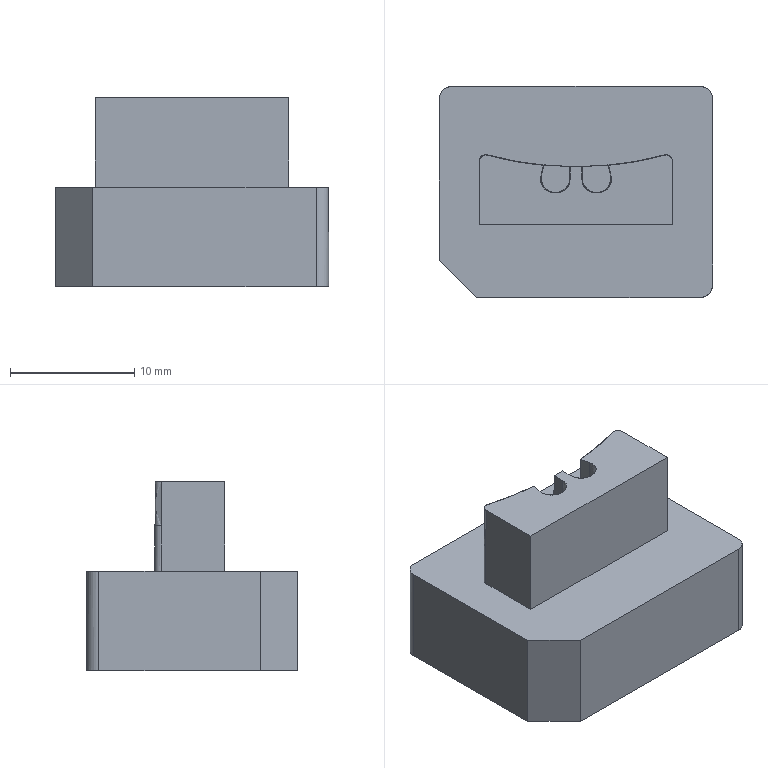NC program | PowerMill | posted by the shop | part box 22 x 17 x 15.232 mm
Lines 11891 to 12632 of 87032:
( TOOL ID   D10_1_1 )
( TOOL DIA. 10. TIP RAD 0 LENGTH 70.4 )
( Z = -.248 )
T3 M6
T10
G91 G28 Z0
G0 G90 G54
M08
S8500 M3
X0 Y0 M8
G43 Z11.802 H3
X-18.215 Y-5.282
Z.952
G1 Z-.248 F360
X-13.104 Y-3.978 F600
X13.103
X13.154 Y-3.766
X13.205 Y-3.487
X13.245 Y-3.182
X13.269 Y-2.829
X13.274 Y-2.625
X13.273 Y.169
X-13.273
Y2.529
X-13.26 Y2.854
X-13.232 Y3.17
X-13.175 Y3.546
X-13.12 Y3.806
X-13.057 Y4.058
X-12.979 Y4.315
X12.979
G0 Z11.802
X0 Y0
Z9.802
X-14.745 Y-16.901
Z-6.23
G1 Z-7.43 F360
X-11.441 Y-12.789 F600
X-1.912 Y-8.025
X-7.919 Y-8.023
X-8.202 Y-8.008
X-8.485 Y-7.978
X-8.768 Y-7.933
X-9.05 Y-7.872
X-9.333 Y-7.795
X-9.616 Y-7.701
X-9.951 Y-7.566
X-10.182 Y-7.458
X-10.464 Y-7.307
X-10.805 Y-7.094
X-11.059 Y-6.911
X-11.313 Y-6.703
X-11.507 Y-6.526
X-11.702 Y-6.33
X-11.879 Y-6.133
X-12.022 Y-5.959
X-12.23 Y-5.675
X-12.444 Y-5.335
X-12.584 Y-5.079
X-12.706 Y-4.824
X-12.823 Y-4.54
X-12.921 Y-4.256
X-13.01 Y-3.945
X-13.068 Y-3.689
X-13.117 Y-3.405
X-13.151 Y-3.121
X-13.17 Y-2.838
X-13.174 Y-2.554
X-13.173 Y2.554
X-13.163 Y2.838
X-13.14 Y3.121
X-13.103 Y3.405
X-13.052 Y3.689
X-13.01 Y3.874
X-12.905 Y4.256
X-12.808 Y4.54
X-12.694 Y4.824
X-12.577 Y5.08
X-12.414 Y5.391
X-12.243 Y5.675
X-12.05 Y5.959
X-11.879 Y6.183
X-11.751 Y6.337
X-11.581 Y6.526
X-11.313 Y6.795
X-11.12 Y6.968
X-10.969 Y7.094
X-10.747 Y7.263
X-10.464 Y7.457
X-10.122 Y7.661
X-9.869 Y7.793
X-9.616 Y7.91
X-9.333 Y8.024
X-9.05 Y8.121
X-8.784 Y8.198
X-8.485 Y8.269
X-8.202 Y8.321
X-7.919 Y8.359
X-7.636 Y8.384
X-7.353 Y8.394
X-7.071 Y8.391
X-6.788 Y8.375
X-6.505 Y8.344
X-6.222 Y8.3
X-5.885 Y8.229
X-5.091 Y8.029
X-4.525 Y7.903
X-3.96 Y7.792
X-3.394 Y7.697
X-2.828 Y7.616
X-2.263 Y7.55
X-1.697 Y7.5
G3 X-.566 Y7.442 I1.713 J22.274
G1 X0 Y7.434
X.566 Y7.442
G3 X1.697 Y7.5 I-.582 J22.332
G1 X2.263 Y7.55
X2.828 Y7.616
X3.394 Y7.697
X3.96 Y7.792
X4.525 Y7.903
X5.091 Y8.029
X5.885 Y8.229
X6.222 Y8.3
X6.505 Y8.344
X6.788 Y8.375
X7.071 Y8.391
X7.353 Y8.394
X7.636 Y8.383
X7.919 Y8.359
X8.202 Y8.321
X8.485 Y8.269
X8.784 Y8.198
X9.05 Y8.121
X9.333 Y8.024
X9.616 Y7.91
X9.839 Y7.808
X10.182 Y7.628
X10.464 Y7.457
X10.747 Y7.263
X10.969 Y7.094
X11.12 Y6.968
X11.313 Y6.795
X11.581 Y6.526
X11.751 Y6.337
X11.879 Y6.183
X12.049 Y5.959
X12.243 Y5.675
X12.444 Y5.336
X12.585 Y5.062
X12.694 Y4.824
X12.808 Y4.54
X12.904 Y4.256
X13.01 Y3.874
X13.052 Y3.689
X13.103 Y3.405
X13.14 Y3.121
X13.163 Y2.838
X13.173 Y2.554
X13.174 Y-2.554
X13.169 Y-2.838
X13.151 Y-3.121
X13.117 Y-3.405
X13.068 Y-3.689
X13.01 Y-3.945
X12.921 Y-4.256
X12.823 Y-4.54
X12.706 Y-4.824
X12.584 Y-5.079
X12.411 Y-5.391
X12.23 Y-5.675
X12.022 Y-5.959
X11.879 Y-6.133
X11.703 Y-6.329
X11.507 Y-6.526
X11.313 Y-6.703
X11.058 Y-6.911
X10.747 Y-7.132
X10.464 Y-7.307
X10.182 Y-7.458
X9.95 Y-7.567
X9.616 Y-7.701
X9.333 Y-7.795
X9.05 Y-7.872
X8.768 Y-7.933
X8.485 Y-7.978
X8.202 Y-8.008
X7.919 Y-8.023
X-1.912 Y-8.025
G0 Z9.802
Z10.802
X0 Y0
X11.833 Y-6.44
Z-6.2
G1 Z-7.4 F360
G3 X10.716 Y-6.704 I-.24 J-1.481 F600
G2 X7.759 Y-7.655 I-2.943 J4.081
G1 X0
X-7.76
G2 X-12.804 Y-2.556 I-.013 J5.032
G1 X-12.803 Y2.558
G2 X-5.913 Y7.855 I5.531 J-.065
G3 X5.185 Y7.671 I5.91 J21.728
G2 X6.1 Y7.898 I19.251 J-75.696
X12.803 Y2.556 I1.174 J-5.403
G1 X12.804 Y-2.556
G2 X10.716 Y-6.704 I-5.031 J-.067
G3 X10.112 Y-7.681 I.877 J-1.217
G1 X11.761 Y-6.402
G3 X10.642 Y-6.658 I-.25 J-1.479
G2 X7.759 Y-7.575 I-2.87 J4.035
G1 X0
X-7.759
G2 X-12.724 Y-2.556 I-.014 J4.952
G1 X-12.723 Y2.556
G2 X-5.933 Y7.777 I5.451 J-.063
G3 X5.203 Y7.593 I5.93 J21.805
G2 X6.116 Y7.819 I19.636 J-77.229
X12.723 Y2.556 I1.159 J-5.325
G1 X12.724 Y-2.556
G2 X10.642 Y-6.658 I-4.951 J-.067
G3 X10.032 Y-7.631 I.869 J-1.222
G0 Z10.802
X0 Y0
Z9.802
X16.348 Y-16.577
Z-14.13
G1 Z-15.33 F360
G3 X13.487 Y-12.476 I-1.43 J2.05 F600
G1 X13.324 Y-12.59
X13.322 Y-12.591
X13.321 Y-12.593
X13.128 Y-12.714
X13.127
X13.126 Y-12.715
X13.002 Y-12.787
X13.001 Y-12.788
X12.999 Y-12.789
X12.683 Y-12.956
X12.682 Y-12.957
X12.68
X12.518 Y-13.034
X12.516 Y-13.035
X12.515
X12.362 Y-13.103
X12.36
X12.359 Y-13.104
X12.043 Y-13.227
X12.04
X12.038 Y-13.228
X11.641 Y-13.354
X11.638 Y-13.355
X11.636 Y-13.356
X11.401 Y-13.416
X11.399 Y-13.417
X11.397
X11.081 Y-13.482
X11.079 Y-13.483
X11.077
X10.761 Y-13.532
X10.759
X10.757 Y-13.533
X10.441 Y-13.563
X10.439 Y-13.564
X10.437
X10.12 Y-13.579
X10.119
X10.117
X9.801 Y-13.58
X-7.904
X-7.905
X-8.221 Y-13.575
X-8.223
X-8.226
X-8.542 Y-13.551
X-8.545
X-8.547 Y-13.55
X-8.863 Y-13.506
X-8.866
X-8.868 Y-13.505
X-9.184 Y-13.44
X-9.187 Y-13.439
X-9.189
X-9.494 Y-13.355
X-9.497
X-9.499 Y-13.354
X-9.827 Y-13.24
X-9.829 Y-13.239
X-9.832 Y-13.238
X-10.148 Y-13.103
X-10.15
X-10.152 Y-13.102
X-10.291 Y-13.034
X-10.293 Y-13.033
X-10.294
X-10.47 Y-12.939
X-10.472 Y-12.938
X-10.474 Y-12.937
X-10.79 Y-12.745
X-10.793 Y-12.743
X-10.796 Y-12.742
X-11.112 Y-12.515
X-11.114 Y-12.514
X-11.115 Y-12.513
X-11.265 Y-12.392
X-11.266 Y-12.391
X-11.267 Y-12.39
X-11.434 Y-12.243
X-11.435 Y-12.242
X-11.437 Y-12.241
X-11.613 Y-12.071
X-11.614
Y-12.07
X-14.599 Y-9.085
X-14.6 Y-9.084
X-14.601 Y-9.083
X-14.768 Y-8.907
X-14.769 Y-8.906
X-14.77 Y-8.904
X-14.919 Y-8.732
X-14.92 Y-8.731
X-14.922 Y-8.729
X-15.035 Y-8.586
X-15.037 Y-8.584
X-15.038 Y-8.582
X-15.24 Y-8.298
X-15.242 Y-8.295
X-15.244 Y-8.293
X-15.453 Y-7.945
X-15.454 Y-7.943
X-15.455 Y-7.94
X-15.562 Y-7.734
X-15.563 Y-7.733
Y-7.732
X-15.616 Y-7.622
Y-7.62
X-15.617 Y-7.618
X-15.75 Y-7.302
X-15.751 Y-7.3
Y-7.297
X-15.859 Y-6.981
X-15.86 Y-6.979
X-15.861 Y-6.976
X-15.946 Y-6.66
Y-6.657
X-15.947 Y-6.655
X-16.01 Y-6.339
X-16.011 Y-6.336
Y-6.334
X-16.054 Y-6.017
Y-6.015
Y-6.012
X-16.076 Y-5.696
Y-5.694
Y-5.692
X-16.08 Y-5.375
Y-5.374
X-16.079 Y7.588
Y7.589
Y7.591
X-16.066 Y7.907
Y7.909
Y7.911
X-16.036 Y8.227
Y8.229
Y8.231
X-15.989 Y8.548
Y8.55
X-15.988 Y8.552
X-15.924 Y8.868
Y8.87
X-15.923 Y8.872
X-15.841 Y9.188
X-15.84 Y9.19
Y9.193
X-15.738 Y9.509
Y9.511
X-15.737 Y9.513
X-15.616 Y9.829
X-15.615 Y9.831
X-15.614 Y9.833
X-15.472 Y10.149
X-15.471 Y10.152
X-15.47 Y10.154
X-15.305 Y10.47
X-15.304 Y10.471
Y10.473
X-15.244 Y10.576
Y10.577
X-15.243 Y10.578
X-15.112 Y10.791
X-15.111 Y10.792
X-15.11 Y10.794
X-14.925 Y11.065
X-14.923 Y11.067
X-14.922 Y11.07
X-14.639 Y11.431
X-14.637 Y11.433
X-14.635 Y11.435
X-14.346 Y11.751
X-14.345 Y11.753
X-14.344 Y11.754
X-14.283 Y11.815
X-14.282 Y11.816
X-14.281 Y11.817
X-14.008 Y12.072
X-14.006 Y12.074
X-14.003 Y12.076
X-13.645 Y12.366
X-13.642 Y12.368
X-13.64 Y12.37
X-13.324 Y12.59
X-13.322 Y12.591
X-13.321 Y12.593
X-13.128 Y12.714
X-13.127
X-13.126 Y12.715
X-13.002 Y12.787
X-13.001 Y12.788
X-12.999 Y12.789
X-12.683 Y12.956
X-12.682 Y12.957
X-12.68
X-12.518 Y13.034
X-12.516 Y13.035
X-12.515
X-12.362 Y13.103
X-12.36
X-12.359 Y13.104
X-12.043 Y13.227
X-12.04
X-12.038 Y13.228
X-11.722 Y13.331
X-11.72 Y13.332
X-11.718
X-11.402 Y13.416
X-11.4 Y13.417
X-11.397
X-11.081 Y13.482
X-11.079 Y13.483
X-11.077
X-10.761 Y13.532
X-10.759
X-10.757 Y13.533
X-10.441 Y13.563
X-10.439 Y13.564
X-10.437
X-10.12 Y13.579
X-10.119
X-10.117
X-9.801 Y13.58
X0
X9.801
X10.117 Y13.579
X10.119
X10.12
X10.436 Y13.564
X10.439
X10.441
X10.757 Y13.533
X10.759 Y13.532
X10.761
X11.077 Y13.484
X11.079 Y13.483
X11.081
X11.398 Y13.417
X11.399
X11.401 Y13.416
X11.636 Y13.356
X11.638 Y13.355
X11.641 Y13.354
X12.038 Y13.228
X12.04 Y13.227
X12.042 Y13.226
X12.359 Y13.104
X12.36 Y13.103
X12.362
X12.515 Y13.035
X12.516
X12.518 Y13.034
X12.68 Y12.957
X12.682 Y12.956
X12.683
X12.999 Y12.789
X13.001 Y12.788
X13.002 Y12.787
X13.126 Y12.715
X13.127 Y12.714
X13.128
X13.321 Y12.593
X13.322 Y12.592
X13.324 Y12.591
X13.606 Y12.395
X13.608 Y12.394
X13.61 Y12.392
X13.96 Y12.113
X13.963 Y12.111
X13.965 Y12.109
X14.281 Y11.817
X14.282 Y11.816
X14.283 Y11.815
X14.344 Y11.754
X14.345 Y11.753
X14.346 Y11.751
X14.602 Y11.473
X14.603 Y11.471
X14.605 Y11.469
X14.888 Y11.115
X14.89 Y11.113
X14.892 Y11.111
X15.11 Y10.794
X15.111 Y10.793
X15.112 Y10.791
X15.243 Y10.578
X15.244 Y10.577
Y10.576
X15.304 Y10.473
Y10.471
X15.305 Y10.47
X15.47 Y10.154
X15.471 Y10.152
X15.472 Y10.149
X15.614 Y9.833
X15.615 Y9.831
X15.616 Y9.829
X15.737 Y9.513
X15.738 Y9.511
X15.739 Y9.509
X15.84 Y9.193
Y9.19
X15.841 Y9.188
X15.923 Y8.872
X15.924 Y8.87
Y8.868
X15.988 Y8.552
Y8.55
Y8.548
X16.036 Y8.232
Y8.229
Y8.227
X16.065 Y7.911
Y7.909
X16.066 Y7.907
X16.079 Y7.591
Y7.589
Y7.587
Y-7.587
Y-7.589
Y-7.591
X16.066 Y-7.907
Y-7.909
Y-7.911
X16.036 Y-8.227
Y-8.229
Y-8.231
X15.989 Y-8.548
Y-8.55
X15.988 Y-8.552
X15.924 Y-8.868
Y-8.87
X15.923 Y-8.872
X15.841 Y-9.188
X15.84 Y-9.19
Y-9.193
X15.738 Y-9.509
Y-9.511
X15.737 Y-9.513
X15.616 Y-9.829
X15.615 Y-9.831
X15.614 Y-9.833
X15.472 Y-10.149
X15.471 Y-10.152
X15.47 Y-10.154
X15.305 Y-10.47
X15.304 Y-10.471
Y-10.473
X15.244 Y-10.576
Y-10.577
X15.243 Y-10.578
X15.112 Y-10.791
X15.111 Y-10.792
X15.11 Y-10.794
X14.925 Y-11.065
X14.923 Y-11.067
X14.922 Y-11.07
X14.639 Y-11.431
X14.637 Y-11.433
X14.635 Y-11.435
X14.346 Y-11.751
X14.345 Y-11.753
X14.344 Y-11.754
X14.283 Y-11.815
X14.282 Y-11.816
X14.281 Y-11.817
X14.008 Y-12.072
X14.006 Y-12.074
X14.003 Y-12.076
X13.645 Y-12.366
X13.642 Y-12.368
X13.64 Y-12.37
X13.487 Y-12.476
G3 X16.348 Y-16.577 I1.43 J-2.05
G1 X16.297 Y-16.515
G3 X13.436 Y-12.415 I-1.43 J2.05
G1 X13.278 Y-12.525
X13.085 Y-12.646
X12.962 Y-12.718
X12.646 Y-12.885
X12.483 Y-12.962
X12.33 Y-13.029
X12.014 Y-13.152
X11.616 Y-13.278
X11.381 Y-13.339
X11.065 Y-13.404
X10.749 Y-13.453
X10.433 Y-13.484
X10.117 Y-13.499
X9.801 Y-13.5
X-7.904
X-8.22 Y-13.495
X-8.536 Y-13.471
X-8.852 Y-13.427
X-9.168 Y-13.362
X-9.473 Y-13.278
X-9.801 Y-13.165
X-10.117 Y-13.03
X-10.256 Y-12.962
X-10.433 Y-12.868
X-10.749 Y-12.677
X-11.065 Y-12.45
X-11.215 Y-12.33
X-11.381 Y-12.183
X-11.558 Y-12.014
X-14.543 Y-9.028
X-14.71 Y-8.852
X-14.859 Y-8.68
X-14.973 Y-8.536
X-15.175 Y-8.251
X-15.384 Y-7.904
X-15.491 Y-7.698
X-15.543 Y-7.587
X-15.676 Y-7.271
X-15.784 Y-6.955
X-15.869 Y-6.639
X-15.932 Y-6.323
X-15.974 Y-6.007
X-15.996 Y-5.691
X-16. Y-5.374
Y7.271
X-15.999 Y7.587
X-15.986 Y7.904
X-15.957 Y8.22
X-15.91 Y8.536
X-15.846 Y8.852
X-15.763 Y9.168
X-15.662 Y9.484
X-15.541 Y9.801
X-15.399 Y10.117
X-15.234 Y10.433
X-15.175 Y10.536
X-15.044 Y10.749
X-14.859 Y11.02
X-14.576 Y11.381
X-14.287 Y11.697
X-14.227 Y11.759
X-13.953 Y12.014
X-13.594 Y12.304
X-13.278 Y12.525
X-13.085 Y12.646
X-12.962 Y12.718
X-12.646 Y12.885
X-12.483 Y12.962
X-12.33 Y13.029
X-12.014 Y13.152
X-11.697 Y13.255
X-11.381 Y13.339
X-11.065 Y13.404
X-10.749 Y13.453
X-10.433 Y13.484
X-10.117 Y13.499
X-9.801 Y13.5
X0
X9.801
X10.117 Y13.499
X10.433 Y13.484
X10.749 Y13.453
X11.065 Y13.405
X11.381 Y13.339
X11.616 Y13.278
X12.014 Y13.152
X12.33 Y13.029
X12.483 Y12.962
X12.646 Y12.885
X12.962 Y12.718
X13.085 Y12.646
X13.278 Y12.525
X13.56 Y12.33
X13.91 Y12.051
X14.227 Y11.759
X14.287 Y11.697
X14.543 Y11.419
X14.826 Y11.065
X15.044 Y10.749
X15.175 Y10.536
X15.234 Y10.433
X15.399 Y10.117
X15.541 Y9.801
X15.662 Y9.484
X15.763 Y9.168
X15.846 Y8.852
X15.909 Y8.536
X15.957 Y8.22
X15.986 Y7.904
X15.999 Y7.587
X16. Y7.271
Y-7.271
X15.999 Y-7.587
X15.986 Y-7.904
X15.957 Y-8.22
X15.91 Y-8.536
X15.846 Y-8.852
X15.763 Y-9.168
X15.662 Y-9.484
X15.541 Y-9.801
X15.399 Y-10.117
X15.234 Y-10.433
X15.175 Y-10.536
X15.044 Y-10.749
X14.859 Y-11.02
X14.576 Y-11.381
X14.287 Y-11.697
X14.227 Y-11.759
X13.953 Y-12.014
X13.594 Y-12.304
X13.436 Y-12.415
G3 X16.297 Y-16.515 I1.43 J-2.05
G0 Z9.802
Z10.802
X0 Y0
M9
M5
M01